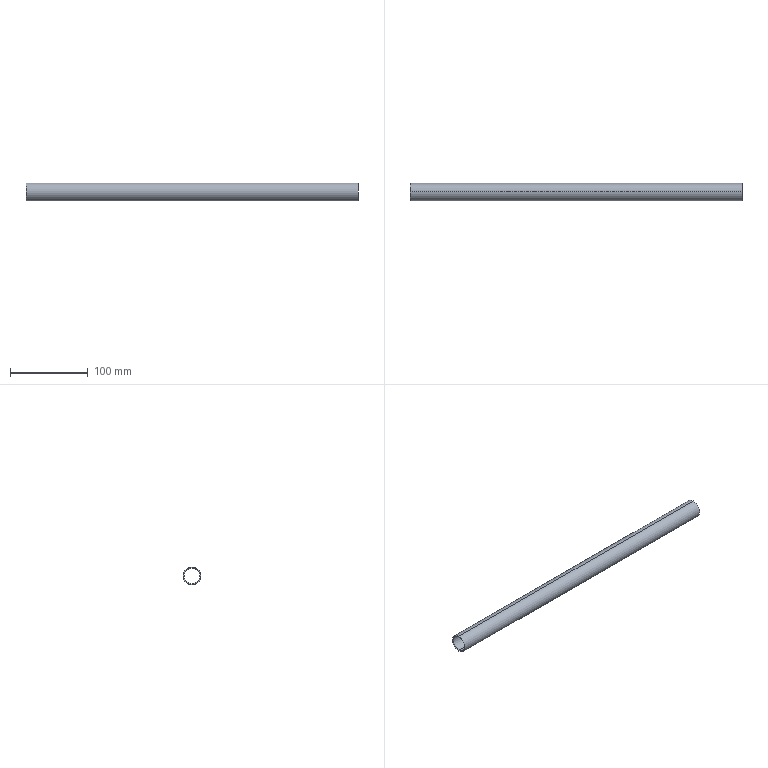Part | STEP file | 1 solid | 10 faces | box 426 x 23 x 23 mm | volume 43129 mm3 | cylinder 4 | cone 4 | plane 2 | commonest cylinder face diameters 20 x2 23 x2
STEP:
#1=CARTESIAN_POINT('',(0.,0.,0.));
#2=DIRECTION('',(0.,0.,1.));
#3=DIRECTION('',(1.,0.,0.));
#4=AXIS2_PLACEMENT_3D('',#1,#2,#3);
#5=CARTESIAN_POINT('',(426.,0.,11.5));
#6=VERTEX_POINT('',#5);
#7=CARTESIAN_POINT('',(426.,0.,-11.5));
#8=VERTEX_POINT('',#7);
#9=CARTESIAN_POINT('',(426.,0.,0.));
#10=DIRECTION('',(-1.,0.,0.));
#11=DIRECTION('',(0.,0.,1.));
#12=AXIS2_PLACEMENT_3D('',#9,#10,#11);
#13=CIRCLE('',#12,11.5);
#14=CARTESIAN_POINT('',(426.,0.,0.));
#15=DIRECTION('',(-1.,0.,0.));
#16=DIRECTION('',(0.,0.,1.));
#17=AXIS2_PLACEMENT_3D('',#14,#15,#16);
#18=CYLINDRICAL_SURFACE('',#17,11.5);
#19=CARTESIAN_POINT('',(0.,0.));
#20=DIRECTION('',(1.,0.));
#21=VECTOR('',#20,1.);
#22=LINE('',#19,#21);
#23=(GEOMETRIC_REPRESENTATION_CONTEXT(2)PARAMETRIC_REPRESENTATION_CONTEXT()REPRESENTATION_CONTEXT('',''));
#24=DEFINITIONAL_REPRESENTATION('',(#22),#23);
#25=PCURVE('',#18,#24);
#26=CARTESIAN_POINT('',(426.,10.707,0.));
#27=DIRECTION('',(-1.,0.,0.));
#28=DIRECTION('',(0.,0.,1.));
#29=AXIS2_PLACEMENT_3D('',#26,#27,#28);
#30=PLANE('',#29);
#31=CARTESIAN_POINT('',(0.,-10.707));
#32=DIRECTION('',(1.,0.));
#33=AXIS2_PLACEMENT_2D('',#31,#32);
#34=CIRCLE('',#33,11.5);
#35=(GEOMETRIC_REPRESENTATION_CONTEXT(2)PARAMETRIC_REPRESENTATION_CONTEXT()REPRESENTATION_CONTEXT('',''));
#36=DEFINITIONAL_REPRESENTATION('',(#34),#35);
#37=PCURVE('',#30,#36);
#38=SURFACE_CURVE('',#13,(#25,#37),.PCURVE_S1.);
#39=EDGE_CURVE('',#6,#8,#38,.T.);
#40=ORIENTED_EDGE('',*,*,#39,.T.);
#41=CARTESIAN_POINT('',(0.,0.,-11.5));
#42=VERTEX_POINT('',#41);
#43=CARTESIAN_POINT('',(426.,0.,-11.5));
#44=DIRECTION('',(-1.,0.,0.));
#45=VECTOR('',#44,1.);
#46=LINE('',#43,#45);
#47=CARTESIAN_POINT('',(3.142,0.));
#48=DIRECTION('',(0.,1.));
#49=VECTOR('',#48,1.);
#50=LINE('',#47,#49);
#51=(GEOMETRIC_REPRESENTATION_CONTEXT(2)PARAMETRIC_REPRESENTATION_CONTEXT()REPRESENTATION_CONTEXT('',''));
#52=DEFINITIONAL_REPRESENTATION('',(#50),#51);
#53=PCURVE('',#18,#52);
#54=CARTESIAN_POINT('',(426.,0.,0.));
#55=DIRECTION('',(-1.,0.,0.));
#56=DIRECTION('',(0.,0.,1.));
#57=AXIS2_PLACEMENT_3D('',#54,#55,#56);
#58=CYLINDRICAL_SURFACE('',#57,11.5);
#59=CARTESIAN_POINT('',(3.142,0.));
#60=DIRECTION('',(0.,1.));
#61=VECTOR('',#60,1.);
#62=LINE('',#59,#61);
#63=(GEOMETRIC_REPRESENTATION_CONTEXT(2)PARAMETRIC_REPRESENTATION_CONTEXT()REPRESENTATION_CONTEXT('',''));
#64=DEFINITIONAL_REPRESENTATION('',(#62),#63);
#65=PCURVE('',#58,#64);
#66=SURFACE_CURVE('',#46,(#53,#65),.PCURVE_S1.);
#67=EDGE_CURVE('',#8,#42,#66,.T.);
#68=ORIENTED_EDGE('',*,*,#67,.T.);
#69=CARTESIAN_POINT('',(0.,0.,11.5));
#70=VERTEX_POINT('',#69);
#71=CARTESIAN_POINT('',(0.,0.,0.));
#72=DIRECTION('',(-1.,0.,0.));
#73=DIRECTION('',(0.,0.,1.));
#74=AXIS2_PLACEMENT_3D('',#71,#72,#73);
#75=CIRCLE('',#74,11.5);
#76=CARTESIAN_POINT('',(0.,426.));
#77=DIRECTION('',(1.,0.));
#78=VECTOR('',#77,1.);
#79=LINE('',#76,#78);
#80=(GEOMETRIC_REPRESENTATION_CONTEXT(2)PARAMETRIC_REPRESENTATION_CONTEXT()REPRESENTATION_CONTEXT('',''));
#81=DEFINITIONAL_REPRESENTATION('',(#79),#80);
#82=PCURVE('',#18,#81);
#83=CARTESIAN_POINT('',(0.,11.5,0.));
#84=DIRECTION('',(1.,0.,0.));
#85=DIRECTION('',(0.,0.,-1.));
#86=AXIS2_PLACEMENT_3D('',#83,#84,#85);
#87=PLANE('',#86);
#88=CARTESIAN_POINT('',(-11.5,-11.5));
#89=CARTESIAN_POINT('',(-11.5,8.419));
#90=CARTESIAN_POINT('',(5.75,-1.541));
#91=CARTESIAN_POINT('',(23.,-11.5));
#92=CARTESIAN_POINT('',(5.75,-21.459));
#93=CARTESIAN_POINT('',(-11.5,-31.419));
#94=CARTESIAN_POINT('',(-11.5,-11.5));
#95=(BOUNDED_CURVE()B_SPLINE_CURVE(2,(#88,#89,#90,#91,#92,#93,#94),.UNSPECIFIED.,.T.,.F.)B_SPLINE_CURVE_WITH_KNOTS((1,2,2,2,2,1),(-2.094,0.,2.094,4.189,6.283,8.378),.UNSPECIFIED.)CURVE()GEOMETRIC_REPRESENTATION_ITEM()RATIONAL_B_SPLINE_CURVE((1.,0.5,1.,0.5,1.,0.5,1.))REPRESENTATION_ITEM(''));
#96=(GEOMETRIC_REPRESENTATION_CONTEXT(2)PARAMETRIC_REPRESENTATION_CONTEXT()REPRESENTATION_CONTEXT('',''));
#97=DEFINITIONAL_REPRESENTATION('',(#95),#96);
#98=PCURVE('',#87,#97);
#99=SURFACE_CURVE('',#75,(#82,#98),.PCURVE_S1.);
#100=EDGE_CURVE('',#70,#42,#99,.T.);
#101=ORIENTED_EDGE('',*,*,#100,.F.);
#102=CARTESIAN_POINT('',(426.,0.,11.5));
#103=DIRECTION('',(-1.,0.,0.));
#104=VECTOR('',#103,1.);
#105=LINE('',#102,#104);
#106=CARTESIAN_POINT('',(0.,0.));
#107=DIRECTION('',(0.,1.));
#108=VECTOR('',#107,1.);
#109=LINE('',#106,#108);
#110=(GEOMETRIC_REPRESENTATION_CONTEXT(2)PARAMETRIC_REPRESENTATION_CONTEXT()REPRESENTATION_CONTEXT('',''));
#111=DEFINITIONAL_REPRESENTATION('',(#109),#110);
#112=PCURVE('',#18,#111);
#113=CARTESIAN_POINT('',(6.283,0.));
#114=DIRECTION('',(0.,1.));
#115=VECTOR('',#114,1.);
#116=LINE('',#113,#115);
#117=(GEOMETRIC_REPRESENTATION_CONTEXT(2)PARAMETRIC_REPRESENTATION_CONTEXT()REPRESENTATION_CONTEXT('',''));
#118=DEFINITIONAL_REPRESENTATION('',(#116),#117);
#119=PCURVE('',#58,#118);
#120=SURFACE_CURVE('',#105,(#112,#119),.PCURVE_S1.);
#121=EDGE_CURVE('',#6,#70,#120,.T.);
#122=ORIENTED_EDGE('',*,*,#121,.F.);
#123=EDGE_LOOP('',(#40,#68,#101,#122));
#124=FACE_BOUND('',#123,.T.);
#125=ADVANCED_FACE('',(#124),#18,.T.);
#126=CARTESIAN_POINT('',(425.293,0.,-10.));
#127=VERTEX_POINT('',#126);
#128=CARTESIAN_POINT('',(426.,0.,-10.707));
#129=VERTEX_POINT('',#128);
#130=CARTESIAN_POINT('',(425.293,0.,-10.));
#131=DIRECTION('',(0.7071,0.,-0.7071));
#132=VECTOR('',#131,1.);
#133=LINE('',#130,#132);
#134=CARTESIAN_POINT('',(425.293,0.,0.));
#135=DIRECTION('',(1.,0.,0.));
#136=DIRECTION('',(0.,0.,-1.));
#137=AXIS2_PLACEMENT_3D('',#134,#135,#136);
#138=CONICAL_SURFACE('',#137,10.,0.7854);
#139=CARTESIAN_POINT('',(6.283,0.));
#140=DIRECTION('',(0.,1.));
#141=VECTOR('',#140,1.);
#142=LINE('',#139,#141);
#143=(GEOMETRIC_REPRESENTATION_CONTEXT(2)PARAMETRIC_REPRESENTATION_CONTEXT()REPRESENTATION_CONTEXT('',''));
#144=DEFINITIONAL_REPRESENTATION('',(#142),#143);
#145=PCURVE('',#138,#144);
#146=CARTESIAN_POINT('',(425.293,0.,0.));
#147=DIRECTION('',(1.,0.,0.));
#148=DIRECTION('',(0.,0.,-1.));
#149=AXIS2_PLACEMENT_3D('',#146,#147,#148);
#150=CONICAL_SURFACE('',#149,10.,0.7854);
#151=CARTESIAN_POINT('',(0.,0.));
#152=DIRECTION('',(0.,1.));
#153=VECTOR('',#152,1.);
#154=LINE('',#151,#153);
#155=(GEOMETRIC_REPRESENTATION_CONTEXT(2)PARAMETRIC_REPRESENTATION_CONTEXT()REPRESENTATION_CONTEXT('',''));
#156=DEFINITIONAL_REPRESENTATION('',(#154),#155);
#157=PCURVE('',#150,#156);
#158=SURFACE_CURVE('',#133,(#145,#157),.PCURVE_S1.);
#159=EDGE_CURVE('',#127,#129,#158,.T.);
#160=ORIENTED_EDGE('',*,*,#159,.T.);
#161=CARTESIAN_POINT('',(426.,0.,10.707));
#162=VERTEX_POINT('',#161);
#163=CARTESIAN_POINT('',(426.,0.,0.));
#164=DIRECTION('',(-1.,0.,0.));
#165=DIRECTION('',(0.,0.,1.));
#166=AXIS2_PLACEMENT_3D('',#163,#164,#165);
#167=CIRCLE('',#166,10.707);
#168=CARTESIAN_POINT('',(9.425,0.7071));
#169=DIRECTION('',(-1.,0.));
#170=VECTOR('',#169,1.);
#171=LINE('',#168,#170);
#172=(GEOMETRIC_REPRESENTATION_CONTEXT(2)PARAMETRIC_REPRESENTATION_CONTEXT()REPRESENTATION_CONTEXT('',''));
#173=DEFINITIONAL_REPRESENTATION('',(#171),#172);
#174=PCURVE('',#138,#173);
#175=CARTESIAN_POINT('',(0.,-10.707));
#176=DIRECTION('',(1.,0.));
#177=AXIS2_PLACEMENT_2D('',#175,#176);
#178=CIRCLE('',#177,10.707);
#179=(GEOMETRIC_REPRESENTATION_CONTEXT(2)PARAMETRIC_REPRESENTATION_CONTEXT()REPRESENTATION_CONTEXT('',''));
#180=DEFINITIONAL_REPRESENTATION('',(#178),#179);
#181=PCURVE('',#30,#180);
#182=SURFACE_CURVE('',#167,(#174,#181),.PCURVE_S1.);
#183=EDGE_CURVE('',#129,#162,#182,.T.);
#184=ORIENTED_EDGE('',*,*,#183,.T.);
#185=CARTESIAN_POINT('',(425.293,0.,10.));
#186=VERTEX_POINT('',#185);
#187=CARTESIAN_POINT('',(425.293,0.,10.));
#188=DIRECTION('',(0.7071,0.,0.7071));
#189=VECTOR('',#188,1.);
#190=LINE('',#187,#189);
#191=CARTESIAN_POINT('',(3.142,0.));
#192=DIRECTION('',(0.,1.));
#193=VECTOR('',#192,1.);
#194=LINE('',#191,#193);
#195=(GEOMETRIC_REPRESENTATION_CONTEXT(2)PARAMETRIC_REPRESENTATION_CONTEXT()REPRESENTATION_CONTEXT('',''));
#196=DEFINITIONAL_REPRESENTATION('',(#194),#195);
#197=PCURVE('',#138,#196);
#198=CARTESIAN_POINT('',(3.142,0.));
#199=DIRECTION('',(0.,1.));
#200=VECTOR('',#199,1.);
#201=LINE('',#198,#200);
#202=(GEOMETRIC_REPRESENTATION_CONTEXT(2)PARAMETRIC_REPRESENTATION_CONTEXT()REPRESENTATION_CONTEXT('',''));
#203=DEFINITIONAL_REPRESENTATION('',(#201),#202);
#204=PCURVE('',#150,#203);
#205=SURFACE_CURVE('',#190,(#197,#204),.PCURVE_S1.);
#206=EDGE_CURVE('',#186,#162,#205,.T.);
#207=ORIENTED_EDGE('',*,*,#206,.F.);
#208=CARTESIAN_POINT('',(425.293,0.,0.));
#209=DIRECTION('',(-1.,0.,0.));
#210=DIRECTION('',(0.,0.,1.));
#211=AXIS2_PLACEMENT_3D('',#208,#209,#210);
#212=CIRCLE('',#211,10.);
#213=CARTESIAN_POINT('',(9.425,0.));
#214=DIRECTION('',(-1.,0.));
#215=VECTOR('',#214,1.);
#216=LINE('',#213,#215);
#217=(GEOMETRIC_REPRESENTATION_CONTEXT(2)PARAMETRIC_REPRESENTATION_CONTEXT()REPRESENTATION_CONTEXT('',''));
#218=DEFINITIONAL_REPRESENTATION('',(#216),#217);
#219=PCURVE('',#138,#218);
#220=CARTESIAN_POINT('',(426.,0.,0.));
#221=DIRECTION('',(-1.,0.,0.));
#222=DIRECTION('',(0.,0.,1.));
#223=AXIS2_PLACEMENT_3D('',#220,#221,#222);
#224=CYLINDRICAL_SURFACE('',#223,10.);
#225=CARTESIAN_POINT('',(0.,0.7071));
#226=DIRECTION('',(1.,0.));
#227=VECTOR('',#226,1.);
#228=LINE('',#225,#227);
#229=(GEOMETRIC_REPRESENTATION_CONTEXT(2)PARAMETRIC_REPRESENTATION_CONTEXT()REPRESENTATION_CONTEXT('',''));
#230=DEFINITIONAL_REPRESENTATION('',(#228),#229);
#231=PCURVE('',#224,#230);
#232=SURFACE_CURVE('',#212,(#219,#231),.PCURVE_S1.);
#233=EDGE_CURVE('',#127,#186,#232,.T.);
#234=ORIENTED_EDGE('',*,*,#233,.F.);
#235=EDGE_LOOP('',(#160,#184,#207,#234));
#236=FACE_BOUND('',#235,.F.);
#237=ADVANCED_FACE('',(#236),#138,.F.);
#238=CARTESIAN_POINT('',(0.7071,0.,10.));
#239=VERTEX_POINT('',#238);
#240=CARTESIAN_POINT('',(426.,0.,10.));
#241=DIRECTION('',(-1.,0.,0.));
#242=VECTOR('',#241,1.);
#243=LINE('',#240,#242);
#244=CARTESIAN_POINT('',(6.283,0.));
#245=DIRECTION('',(0.,1.));
#246=VECTOR('',#245,1.);
#247=LINE('',#244,#246);
#248=(GEOMETRIC_REPRESENTATION_CONTEXT(2)PARAMETRIC_REPRESENTATION_CONTEXT()REPRESENTATION_CONTEXT('',''));
#249=DEFINITIONAL_REPRESENTATION('',(#247),#248);
#250=PCURVE('',#224,#249);
#251=CARTESIAN_POINT('',(426.,0.,0.));
#252=DIRECTION('',(-1.,0.,0.));
#253=DIRECTION('',(0.,0.,1.));
#254=AXIS2_PLACEMENT_3D('',#251,#252,#253);
#255=CYLINDRICAL_SURFACE('',#254,10.);
#256=CARTESIAN_POINT('',(0.,0.));
#257=DIRECTION('',(0.,1.));
#258=VECTOR('',#257,1.);
#259=LINE('',#256,#258);
#260=(GEOMETRIC_REPRESENTATION_CONTEXT(2)PARAMETRIC_REPRESENTATION_CONTEXT()REPRESENTATION_CONTEXT('',''));
#261=DEFINITIONAL_REPRESENTATION('',(#259),#260);
#262=PCURVE('',#255,#261);
#263=SURFACE_CURVE('',#243,(#250,#262),.PCURVE_S1.);
#264=EDGE_CURVE('',#186,#239,#263,.T.);
#265=ORIENTED_EDGE('',*,*,#264,.T.);
#266=CARTESIAN_POINT('',(0.7071,0.,-10.));
#267=VERTEX_POINT('',#266);
#268=CARTESIAN_POINT('',(0.7071,0.,0.));
#269=DIRECTION('',(-1.,0.,0.));
#270=DIRECTION('',(0.,0.,1.));
#271=AXIS2_PLACEMENT_3D('',#268,#269,#270);
#272=CIRCLE('',#271,10.);
#273=CARTESIAN_POINT('',(0.,425.293));
#274=DIRECTION('',(1.,0.));
#275=VECTOR('',#274,1.);
#276=LINE('',#273,#275);
#277=(GEOMETRIC_REPRESENTATION_CONTEXT(2)PARAMETRIC_REPRESENTATION_CONTEXT()REPRESENTATION_CONTEXT('',''));
#278=DEFINITIONAL_REPRESENTATION('',(#276),#277);
#279=PCURVE('',#224,#278);
#280=CARTESIAN_POINT('',(0.,0.,0.));
#281=DIRECTION('',(-1.,0.,0.));
#282=DIRECTION('',(0.,0.,1.));
#283=AXIS2_PLACEMENT_3D('',#280,#281,#282);
#284=CONICAL_SURFACE('',#283,10.707,0.7854);
#285=CARTESIAN_POINT('',(0.,-0.7071));
#286=DIRECTION('',(1.,0.));
#287=VECTOR('',#286,1.);
#288=LINE('',#285,#287);
#289=(GEOMETRIC_REPRESENTATION_CONTEXT(2)PARAMETRIC_REPRESENTATION_CONTEXT()REPRESENTATION_CONTEXT('',''));
#290=DEFINITIONAL_REPRESENTATION('',(#288),#289);
#291=PCURVE('',#284,#290);
#292=SURFACE_CURVE('',#272,(#279,#291),.PCURVE_S1.);
#293=EDGE_CURVE('',#267,#239,#292,.T.);
#294=ORIENTED_EDGE('',*,*,#293,.F.);
#295=CARTESIAN_POINT('',(426.,0.,-10.));
#296=DIRECTION('',(-1.,0.,0.));
#297=VECTOR('',#296,1.);
#298=LINE('',#295,#297);
#299=CARTESIAN_POINT('',(3.142,0.));
#300=DIRECTION('',(0.,1.));
#301=VECTOR('',#300,1.);
#302=LINE('',#299,#301);
#303=(GEOMETRIC_REPRESENTATION_CONTEXT(2)PARAMETRIC_REPRESENTATION_CONTEXT()REPRESENTATION_CONTEXT('',''));
#304=DEFINITIONAL_REPRESENTATION('',(#302),#303);
#305=PCURVE('',#224,#304);
#306=CARTESIAN_POINT('',(3.142,0.));
#307=DIRECTION('',(0.,1.));
#308=VECTOR('',#307,1.);
#309=LINE('',#306,#308);
#310=(GEOMETRIC_REPRESENTATION_CONTEXT(2)PARAMETRIC_REPRESENTATION_CONTEXT()REPRESENTATION_CONTEXT('',''));
#311=DEFINITIONAL_REPRESENTATION('',(#309),#310);
#312=PCURVE('',#255,#311);
#313=SURFACE_CURVE('',#298,(#305,#312),.PCURVE_S1.);
#314=EDGE_CURVE('',#127,#267,#313,.T.);
#315=ORIENTED_EDGE('',*,*,#314,.F.);
#316=ORIENTED_EDGE('',*,*,#233,.T.);
#317=EDGE_LOOP('',(#265,#294,#315,#316));
#318=FACE_BOUND('',#317,.F.);
#319=ADVANCED_FACE('',(#318),#224,.F.);
#320=CARTESIAN_POINT('',(0.,0.,10.707));
#321=VERTEX_POINT('',#320);
#322=CARTESIAN_POINT('',(0.,0.,10.707));
#323=DIRECTION('',(-0.7071,0.,0.7071));
#324=VECTOR('',#323,1.);
#325=LINE('',#322,#324);
#326=CARTESIAN_POINT('',(6.283,0.));
#327=DIRECTION('',(0.,1.));
#328=VECTOR('',#327,1.);
#329=LINE('',#326,#328);
#330=(GEOMETRIC_REPRESENTATION_CONTEXT(2)PARAMETRIC_REPRESENTATION_CONTEXT()REPRESENTATION_CONTEXT('',''));
#331=DEFINITIONAL_REPRESENTATION('',(#329),#330);
#332=PCURVE('',#284,#331);
#333=CARTESIAN_POINT('',(0.,0.,0.));
#334=DIRECTION('',(-1.,0.,0.));
#335=DIRECTION('',(0.,0.,1.));
#336=AXIS2_PLACEMENT_3D('',#333,#334,#335);
#337=CONICAL_SURFACE('',#336,10.707,0.7854);
#338=CARTESIAN_POINT('',(0.,0.));
#339=DIRECTION('',(0.,1.));
#340=VECTOR('',#339,1.);
#341=LINE('',#338,#340);
#342=(GEOMETRIC_REPRESENTATION_CONTEXT(2)PARAMETRIC_REPRESENTATION_CONTEXT()REPRESENTATION_CONTEXT('',''));
#343=DEFINITIONAL_REPRESENTATION('',(#341),#342);
#344=PCURVE('',#337,#343);
#345=SURFACE_CURVE('',#325,(#332,#344),.PCURVE_S1.);
#346=EDGE_CURVE('',#239,#321,#345,.T.);
#347=ORIENTED_EDGE('',*,*,#346,.T.);
#348=CARTESIAN_POINT('',(0.,0.,-10.707));
#349=VERTEX_POINT('',#348);
#350=CARTESIAN_POINT('',(0.,0.,0.));
#351=DIRECTION('',(-1.,0.,0.));
#352=DIRECTION('',(0.,0.,1.));
#353=AXIS2_PLACEMENT_3D('',#350,#351,#352);
#354=CIRCLE('',#353,10.707);
#355=CARTESIAN_POINT('',(0.,0.));
#356=DIRECTION('',(1.,0.));
#357=VECTOR('',#356,1.);
#358=LINE('',#355,#357);
#359=(GEOMETRIC_REPRESENTATION_CONTEXT(2)PARAMETRIC_REPRESENTATION_CONTEXT()REPRESENTATION_CONTEXT('',''));
#360=DEFINITIONAL_REPRESENTATION('',(#358),#359);
#361=PCURVE('',#284,#360);
#362=CARTESIAN_POINT('',(-10.707,-11.5));
#363=CARTESIAN_POINT('',(-10.707,7.045));
#364=CARTESIAN_POINT('',(5.354,-2.227));
#365=CARTESIAN_POINT('',(21.414,-11.5));
#366=CARTESIAN_POINT('',(5.354,-20.773));
#367=CARTESIAN_POINT('',(-10.707,-30.045));
#368=CARTESIAN_POINT('',(-10.707,-11.5));
#369=(BOUNDED_CURVE()B_SPLINE_CURVE(2,(#362,#363,#364,#365,#366,#367,#368),.UNSPECIFIED.,.T.,.F.)B_SPLINE_CURVE_WITH_KNOTS((1,2,2,2,2,1),(-2.094,0.,2.094,4.189,6.283,8.378),.UNSPECIFIED.)CURVE()GEOMETRIC_REPRESENTATION_ITEM()RATIONAL_B_SPLINE_CURVE((1.,0.5,1.,0.5,1.,0.5,1.))REPRESENTATION_ITEM(''));
#370=(GEOMETRIC_REPRESENTATION_CONTEXT(2)PARAMETRIC_REPRESENTATION_CONTEXT()REPRESENTATION_CONTEXT('',''));
#371=DEFINITIONAL_REPRESENTATION('',(#369),#370);
#372=PCURVE('',#87,#371);
#373=SURFACE_CURVE('',#354,(#361,#372),.PCURVE_S1.);
#374=EDGE_CURVE('',#349,#321,#373,.T.);
#375=ORIENTED_EDGE('',*,*,#374,.F.);
#376=CARTESIAN_POINT('',(0.,0.,-10.707));
#377=DIRECTION('',(-0.7071,0.,-0.7071));
#378=VECTOR('',#377,1.);
#379=LINE('',#376,#378);
#380=CARTESIAN_POINT('',(3.142,0.));
#381=DIRECTION('',(0.,1.));
#382=VECTOR('',#381,1.);
#383=LINE('',#380,#382);
#384=(GEOMETRIC_REPRESENTATION_CONTEXT(2)PARAMETRIC_REPRESENTATION_CONTEXT()REPRESENTATION_CONTEXT('',''));
#385=DEFINITIONAL_REPRESENTATION('',(#383),#384);
#386=PCURVE('',#284,#385);
#387=CARTESIAN_POINT('',(3.142,0.));
#388=DIRECTION('',(0.,1.));
#389=VECTOR('',#388,1.);
#390=LINE('',#387,#389);
#391=(GEOMETRIC_REPRESENTATION_CONTEXT(2)PARAMETRIC_REPRESENTATION_CONTEXT()REPRESENTATION_CONTEXT('',''));
#392=DEFINITIONAL_REPRESENTATION('',(#390),#391);
#393=PCURVE('',#337,#392);
#394=SURFACE_CURVE('',#379,(#386,#393),.PCURVE_S1.);
#395=EDGE_CURVE('',#267,#349,#394,.T.);
#396=ORIENTED_EDGE('',*,*,#395,.F.);
#397=ORIENTED_EDGE('',*,*,#293,.T.);
#398=EDGE_LOOP('',(#347,#375,#396,#397));
#399=FACE_BOUND('',#398,.F.);
#400=ADVANCED_FACE('',(#399),#284,.F.);
#401=CARTESIAN_POINT('',(0.,0.,0.));
#402=DIRECTION('',(-1.,0.,0.));
#403=DIRECTION('',(0.,0.,1.));
#404=AXIS2_PLACEMENT_3D('',#401,#402,#403);
#405=CIRCLE('',#404,10.707);
#406=CARTESIAN_POINT('',(-10.707,-11.5));
#407=CARTESIAN_POINT('',(-10.707,7.045));
#408=CARTESIAN_POINT('',(5.354,-2.227));
#409=CARTESIAN_POINT('',(21.414,-11.5));
#410=CARTESIAN_POINT('',(5.354,-20.773));
#411=CARTESIAN_POINT('',(-10.707,-30.045));
#412=CARTESIAN_POINT('',(-10.707,-11.5));
#413=(BOUNDED_CURVE()B_SPLINE_CURVE(2,(#406,#407,#408,#409,#410,#411,#412),.UNSPECIFIED.,.T.,.F.)B_SPLINE_CURVE_WITH_KNOTS((1,2,2,2,2,1),(-2.094,0.,2.094,4.189,6.283,8.378),.UNSPECIFIED.)CURVE()GEOMETRIC_REPRESENTATION_ITEM()RATIONAL_B_SPLINE_CURVE((1.,0.5,1.,0.5,1.,0.5,1.))REPRESENTATION_ITEM(''));
#414=(GEOMETRIC_REPRESENTATION_CONTEXT(2)PARAMETRIC_REPRESENTATION_CONTEXT()REPRESENTATION_CONTEXT('',''));
#415=DEFINITIONAL_REPRESENTATION('',(#413),#414);
#416=PCURVE('',#87,#415);
#417=CARTESIAN_POINT('',(0.,0.));
#418=DIRECTION('',(1.,0.));
#419=VECTOR('',#418,1.);
#420=LINE('',#417,#419);
#421=(GEOMETRIC_REPRESENTATION_CONTEXT(2)PARAMETRIC_REPRESENTATION_CONTEXT()REPRESENTATION_CONTEXT('',''));
#422=DEFINITIONAL_REPRESENTATION('',(#420),#421);
#423=PCURVE('',#337,#422);
#424=SURFACE_CURVE('',#405,(#416,#423),.PCURVE_S1.);
#425=EDGE_CURVE('',#321,#349,#424,.T.);
#426=ORIENTED_EDGE('',*,*,#425,.F.);
#427=ORIENTED_EDGE('',*,*,#374,.F.);
#428=EDGE_LOOP('',(#426,#427));
#429=FACE_BOUND('',#428,.T.);
#430=ORIENTED_EDGE('',*,*,#100,.T.);
#431=CARTESIAN_POINT('',(0.,0.,0.));
#432=DIRECTION('',(-1.,0.,0.));
#433=DIRECTION('',(0.,0.,1.));
#434=AXIS2_PLACEMENT_3D('',#431,#432,#433);
#435=CIRCLE('',#434,11.5);
#436=CARTESIAN_POINT('',(-11.5,-11.5));
#437=CARTESIAN_POINT('',(-11.5,8.419));
#438=CARTESIAN_POINT('',(5.75,-1.541));
#439=CARTESIAN_POINT('',(23.,-11.5));
#440=CARTESIAN_POINT('',(5.75,-21.459));
#441=CARTESIAN_POINT('',(-11.5,-31.419));
#442=CARTESIAN_POINT('',(-11.5,-11.5));
#443=(BOUNDED_CURVE()B_SPLINE_CURVE(2,(#436,#437,#438,#439,#440,#441,#442),.UNSPECIFIED.,.T.,.F.)B_SPLINE_CURVE_WITH_KNOTS((1,2,2,2,2,1),(-2.094,0.,2.094,4.189,6.283,8.378),.UNSPECIFIED.)CURVE()GEOMETRIC_REPRESENTATION_ITEM()RATIONAL_B_SPLINE_CURVE((1.,0.5,1.,0.5,1.,0.5,1.))REPRESENTATION_ITEM(''));
#444=(GEOMETRIC_REPRESENTATION_CONTEXT(2)PARAMETRIC_REPRESENTATION_CONTEXT()REPRESENTATION_CONTEXT('',''));
#445=DEFINITIONAL_REPRESENTATION('',(#443),#444);
#446=PCURVE('',#87,#445);
#447=CARTESIAN_POINT('',(0.,426.));
#448=DIRECTION('',(1.,0.));
#449=VECTOR('',#448,1.);
#450=LINE('',#447,#449);
#451=(GEOMETRIC_REPRESENTATION_CONTEXT(2)PARAMETRIC_REPRESENTATION_CONTEXT()REPRESENTATION_CONTEXT('',''));
#452=DEFINITIONAL_REPRESENTATION('',(#450),#451);
#453=PCURVE('',#58,#452);
#454=SURFACE_CURVE('',#435,(#446,#453),.PCURVE_S1.);
#455=EDGE_CURVE('',#42,#70,#454,.T.);
#456=ORIENTED_EDGE('',*,*,#455,.T.);
#457=EDGE_LOOP('',(#430,#456));
#458=FACE_BOUND('',#457,.T.);
#459=ADVANCED_FACE('',(#429,#458),#87,.F.);
#460=ORIENTED_EDGE('',*,*,#425,.F.);
#461=ORIENTED_EDGE('',*,*,#346,.F.);
#462=CARTESIAN_POINT('',(0.7071,0.,0.));
#463=DIRECTION('',(-1.,0.,0.));
#464=DIRECTION('',(0.,0.,1.));
#465=AXIS2_PLACEMENT_3D('',#462,#463,#464);
#466=CIRCLE('',#465,10.);
#467=CARTESIAN_POINT('',(0.,-0.7071));
#468=DIRECTION('',(1.,0.));
#469=VECTOR('',#468,1.);
#470=LINE('',#467,#469);
#471=(GEOMETRIC_REPRESENTATION_CONTEXT(2)PARAMETRIC_REPRESENTATION_CONTEXT()REPRESENTATION_CONTEXT('',''));
#472=DEFINITIONAL_REPRESENTATION('',(#470),#471);
#473=PCURVE('',#337,#472);
#474=CARTESIAN_POINT('',(0.,425.293));
#475=DIRECTION('',(1.,0.));
#476=VECTOR('',#475,1.);
#477=LINE('',#474,#476);
#478=(GEOMETRIC_REPRESENTATION_CONTEXT(2)PARAMETRIC_REPRESENTATION_CONTEXT()REPRESENTATION_CONTEXT('',''));
#479=DEFINITIONAL_REPRESENTATION('',(#477),#478);
#480=PCURVE('',#255,#479);
#481=SURFACE_CURVE('',#466,(#473,#480),.PCURVE_S1.);
#482=EDGE_CURVE('',#239,#267,#481,.T.);
#483=ORIENTED_EDGE('',*,*,#482,.T.);
#484=ORIENTED_EDGE('',*,*,#395,.T.);
#485=EDGE_LOOP('',(#460,#461,#483,#484));
#486=FACE_BOUND('',#485,.F.);
#487=ADVANCED_FACE('',(#486),#337,.F.);
#488=ORIENTED_EDGE('',*,*,#482,.F.);
#489=ORIENTED_EDGE('',*,*,#264,.F.);
#490=CARTESIAN_POINT('',(425.293,0.,0.));
#491=DIRECTION('',(-1.,0.,0.));
#492=DIRECTION('',(0.,0.,1.));
#493=AXIS2_PLACEMENT_3D('',#490,#491,#492);
#494=CIRCLE('',#493,10.);
#495=CARTESIAN_POINT('',(0.,0.7071));
#496=DIRECTION('',(1.,0.));
#497=VECTOR('',#496,1.);
#498=LINE('',#495,#497);
#499=(GEOMETRIC_REPRESENTATION_CONTEXT(2)PARAMETRIC_REPRESENTATION_CONTEXT()REPRESENTATION_CONTEXT('',''));
#500=DEFINITIONAL_REPRESENTATION('',(#498),#499);
#501=PCURVE('',#255,#500);
#502=CARTESIAN_POINT('',(3.142,0.));
#503=DIRECTION('',(-1.,0.));
#504=VECTOR('',#503,1.);
#505=LINE('',#502,#504);
#506=(GEOMETRIC_REPRESENTATION_CONTEXT(2)PARAMETRIC_REPRESENTATION_CONTEXT()REPRESENTATION_CONTEXT('',''));
#507=DEFINITIONAL_REPRESENTATION('',(#505),#506);
#508=PCURVE('',#150,#507);
#509=SURFACE_CURVE('',#494,(#501,#508),.PCURVE_S1.);
#510=EDGE_CURVE('',#186,#127,#509,.T.);
#511=ORIENTED_EDGE('',*,*,#510,.T.);
#512=ORIENTED_EDGE('',*,*,#314,.T.);
#513=EDGE_LOOP('',(#488,#489,#511,#512));
#514=FACE_BOUND('',#513,.F.);
#515=ADVANCED_FACE('',(#514),#255,.F.);
#516=CARTESIAN_POINT('',(426.,0.,0.));
#517=DIRECTION('',(-1.,0.,0.));
#518=DIRECTION('',(0.,0.,1.));
#519=AXIS2_PLACEMENT_3D('',#516,#517,#518);
#520=CIRCLE('',#519,10.707);
#521=CARTESIAN_POINT('',(3.142,0.7071));
#522=DIRECTION('',(-1.,0.));
#523=VECTOR('',#522,1.);
#524=LINE('',#521,#523);
#525=(GEOMETRIC_REPRESENTATION_CONTEXT(2)PARAMETRIC_REPRESENTATION_CONTEXT()REPRESENTATION_CONTEXT('',''));
#526=DEFINITIONAL_REPRESENTATION('',(#524),#525);
#527=PCURVE('',#150,#526);
#528=CARTESIAN_POINT('',(0.,-10.707));
#529=DIRECTION('',(1.,0.));
#530=AXIS2_PLACEMENT_2D('',#528,#529);
#531=CIRCLE('',#530,10.707);
#532=(GEOMETRIC_REPRESENTATION_CONTEXT(2)PARAMETRIC_REPRESENTATION_CONTEXT()REPRESENTATION_CONTEXT('',''));
#533=DEFINITIONAL_REPRESENTATION('',(#531),#532);
#534=PCURVE('',#30,#533);
#535=SURFACE_CURVE('',#520,(#527,#534),.PCURVE_S1.);
#536=EDGE_CURVE('',#162,#129,#535,.T.);
#537=ORIENTED_EDGE('',*,*,#536,.T.);
#538=ORIENTED_EDGE('',*,*,#159,.F.);
#539=ORIENTED_EDGE('',*,*,#510,.F.);
#540=ORIENTED_EDGE('',*,*,#206,.T.);
#541=EDGE_LOOP('',(#537,#538,#539,#540));
#542=FACE_BOUND('',#541,.F.);
#543=ADVANCED_FACE('',(#542),#150,.F.);
#544=ORIENTED_EDGE('',*,*,#39,.F.);
#545=CARTESIAN_POINT('',(426.,0.,0.));
#546=DIRECTION('',(-1.,0.,0.));
#547=DIRECTION('',(0.,0.,1.));
#548=AXIS2_PLACEMENT_3D('',#545,#546,#547);
#549=CIRCLE('',#548,11.5);
#550=CARTESIAN_POINT('',(0.,-10.707));
#551=DIRECTION('',(1.,0.));
#552=AXIS2_PLACEMENT_2D('',#550,#551);
#553=CIRCLE('',#552,11.5);
#554=(GEOMETRIC_REPRESENTATION_CONTEXT(2)PARAMETRIC_REPRESENTATION_CONTEXT()REPRESENTATION_CONTEXT('',''));
#555=DEFINITIONAL_REPRESENTATION('',(#553),#554);
#556=PCURVE('',#30,#555);
#557=CARTESIAN_POINT('',(0.,0.));
#558=DIRECTION('',(1.,0.));
#559=VECTOR('',#558,1.);
#560=LINE('',#557,#559);
#561=(GEOMETRIC_REPRESENTATION_CONTEXT(2)PARAMETRIC_REPRESENTATION_CONTEXT()REPRESENTATION_CONTEXT('',''));
#562=DEFINITIONAL_REPRESENTATION('',(#560),#561);
#563=PCURVE('',#58,#562);
#564=SURFACE_CURVE('',#549,(#556,#563),.PCURVE_S1.);
#565=EDGE_CURVE('',#8,#6,#564,.T.);
#566=ORIENTED_EDGE('',*,*,#565,.F.);
#567=EDGE_LOOP('',(#544,#566));
#568=FACE_BOUND('',#567,.T.);
#569=ORIENTED_EDGE('',*,*,#183,.T.);
#570=ORIENTED_EDGE('',*,*,#536,.T.);
#571=EDGE_LOOP('',(#569,#570));
#572=FACE_BOUND('',#571,.T.);
#573=ADVANCED_FACE('',(#568,#572),#30,.F.);
#574=ORIENTED_EDGE('',*,*,#67,.F.);
#575=ORIENTED_EDGE('',*,*,#565,.T.);
#576=ORIENTED_EDGE('',*,*,#121,.T.);
#577=ORIENTED_EDGE('',*,*,#455,.F.);
#578=EDGE_LOOP('',(#574,#575,#576,#577));
#579=FACE_BOUND('',#578,.T.);
#580=ADVANCED_FACE('',(#579),#58,.T.);
#581=CLOSED_SHELL('',(#125,#237,#319,#400,#459,#487,#515,#543,#573,#580));
#582=MANIFOLD_SOLID_BREP('',#581);
#583=(LENGTH_UNIT()NAMED_UNIT(*)SI_UNIT(.MILLI.,.METRE.));
#584=UNCERTAINTY_MEASURE_WITH_UNIT(LENGTH_MEASURE(0.0000001),#583,'','');
#585=(NAMED_UNIT(*)PLANE_ANGLE_UNIT()SI_UNIT($,.RADIAN.));
#586=(NAMED_UNIT(*)SI_UNIT($,.STERADIAN.)SOLID_ANGLE_UNIT());
#587=(GEOMETRIC_REPRESENTATION_CONTEXT(3)GLOBAL_UNCERTAINTY_ASSIGNED_CONTEXT((#584))GLOBAL_UNIT_ASSIGNED_CONTEXT((#583,#585,#586))REPRESENTATION_CONTEXT('',''));
#588=ADVANCED_BREP_SHAPE_REPRESENTATION('',(#4,#582),#587);